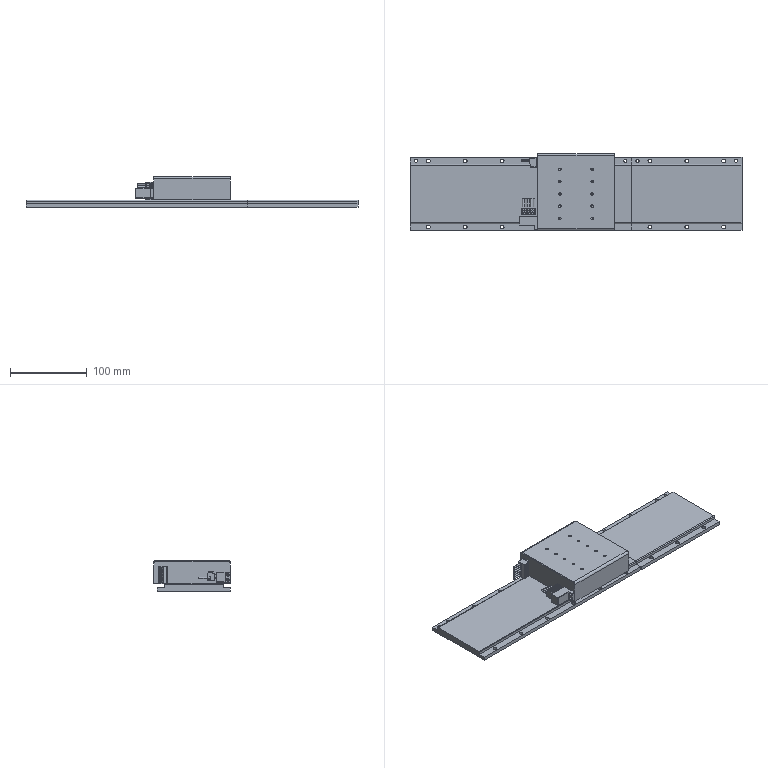Part | NX | features BREP 12 | 12 solids | 800 faces | box 431.8 x 100 x 40 mm | volume 648515 mm3 | plane 563 | cylinder 177 | cone 60 | commonest cylinder face diameters 4.8 x36 1.404 x22 2.01 x22 2.8 x22 3.242 x20 0.5 x12